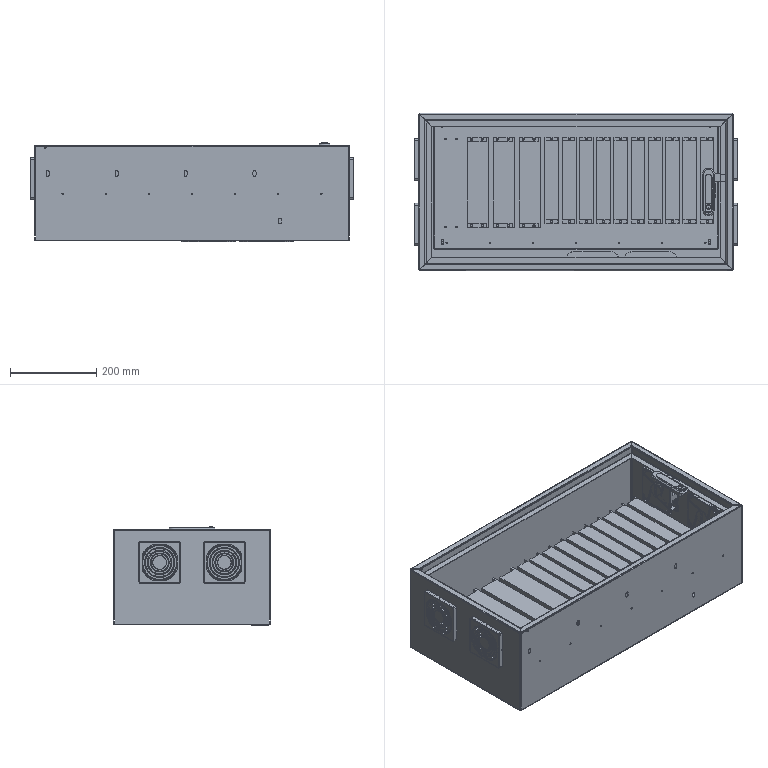Part | SolidWorks | features ReferencePattern 24, InContextFeatHolder 4, LocalLPattern 3, CompositeCurve 1 | 38 solids | 6833 faces | volume 11450307 mm3 | plane 4028 | cylinder 1750 | torus 668 | spline 170 | cone 165 | sphere 52 | commonest cylinder face diameters 1 x252 2 x202 3.3 x142 4.8 x116 0.6 x76 90 x76